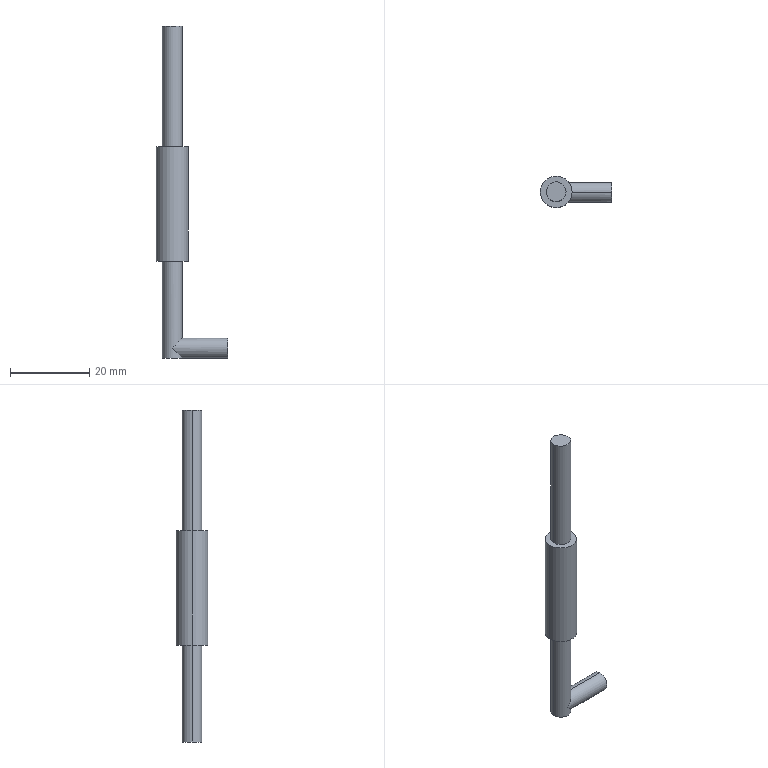Part | STEP file | HI_HFG87-17-002(2)^HFG87-17(2)_Lower机架DoorPlate 2 | 1 solid | 13 faces | box 18 x 8 x 84 mm | volume 2771 mm3 | cylinder 8 | plane 5 | commonest cylinder face diameters 5 x6 8 x2
STEP:
#1=CARTESIAN_POINT('',(0.,0.,0.));
#2=DIRECTION('',(0.,0.,1.));
#3=DIRECTION('',(1.,0.,0.));
#4=AXIS2_PLACEMENT_3D('',#1,#2,#3);
#5=CARTESIAN_POINT('',(-2.5,0.,44.5));
#6=VERTEX_POINT('',#5);
#7=CARTESIAN_POINT('',(2.5,0.,44.5));
#8=VERTEX_POINT('',#7);
#9=CARTESIAN_POINT('',(0.,0.,44.5));
#10=DIRECTION('',(0.,0.,1.));
#11=DIRECTION('',(1.,0.,0.));
#12=AXIS2_PLACEMENT_3D('',#9,#10,#11);
#13=CIRCLE('',#12,2.5);
#14=CARTESIAN_POINT('',(0.,0.,75.));
#15=DIRECTION('',(0.,0.,1.));
#16=DIRECTION('',(-1.,0.,0.));
#17=AXIS2_PLACEMENT_3D('',#14,#15,#16);
#18=CYLINDRICAL_SURFACE('',#17,2.5);
#19=CARTESIAN_POINT('',(-3.142,-30.5));
#20=DIRECTION('',(1.,0.));
#21=VECTOR('',#20,1.);
#22=LINE('',#19,#21);
#23=(GEOMETRIC_REPRESENTATION_CONTEXT(2)PARAMETRIC_REPRESENTATION_CONTEXT()REPRESENTATION_CONTEXT('',''));
#24=DEFINITIONAL_REPRESENTATION('',(#22),#23);
#25=PCURVE('',#18,#24);
#26=CARTESIAN_POINT('',(0.,0.,44.5));
#27=DIRECTION('',(0.,0.,1.));
#28=DIRECTION('',(1.,0.,0.));
#29=AXIS2_PLACEMENT_3D('',#26,#27,#28);
#30=PLANE('',#29);
#31=CARTESIAN_POINT('',(0.,0.));
#32=DIRECTION('',(1.,0.));
#33=AXIS2_PLACEMENT_2D('',#31,#32);
#34=CIRCLE('',#33,2.5);
#35=(GEOMETRIC_REPRESENTATION_CONTEXT(2)PARAMETRIC_REPRESENTATION_CONTEXT()REPRESENTATION_CONTEXT('',''));
#36=DEFINITIONAL_REPRESENTATION('',(#34),#35);
#37=PCURVE('',#30,#36);
#38=SURFACE_CURVE('',#13,(#25,#37),.PCURVE_S1.);
#39=EDGE_CURVE('',#6,#8,#38,.T.);
#40=ORIENTED_EDGE('',*,*,#39,.T.);
#41=CARTESIAN_POINT('',(2.5,0.,75.));
#42=VERTEX_POINT('',#41);
#43=CARTESIAN_POINT('',(2.5,0.,75.));
#44=DIRECTION('',(0.,0.,1.));
#45=VECTOR('',#44,1.);
#46=LINE('',#43,#45);
#47=CARTESIAN_POINT('',(3.142,0.));
#48=DIRECTION('',(0.,1.));
#49=VECTOR('',#48,1.);
#50=LINE('',#47,#49);
#51=(GEOMETRIC_REPRESENTATION_CONTEXT(2)PARAMETRIC_REPRESENTATION_CONTEXT()REPRESENTATION_CONTEXT('',''));
#52=DEFINITIONAL_REPRESENTATION('',(#50),#51);
#53=PCURVE('',#18,#52);
#54=CARTESIAN_POINT('',(0.,0.,75.));
#55=DIRECTION('',(0.,0.,1.));
#56=DIRECTION('',(-1.,0.,0.));
#57=AXIS2_PLACEMENT_3D('',#54,#55,#56);
#58=CYLINDRICAL_SURFACE('',#57,2.5);
#59=CARTESIAN_POINT('',(3.142,0.));
#60=DIRECTION('',(0.,1.));
#61=VECTOR('',#60,1.);
#62=LINE('',#59,#61);
#63=(GEOMETRIC_REPRESENTATION_CONTEXT(2)PARAMETRIC_REPRESENTATION_CONTEXT()REPRESENTATION_CONTEXT('',''));
#64=DEFINITIONAL_REPRESENTATION('',(#62),#63);
#65=PCURVE('',#58,#64);
#66=SURFACE_CURVE('',#46,(#53,#65),.PCURVE_S1.);
#67=EDGE_CURVE('',#8,#42,#66,.T.);
#68=ORIENTED_EDGE('',*,*,#67,.T.);
#69=CARTESIAN_POINT('',(-2.5,0.,75.));
#70=VERTEX_POINT('',#69);
#71=CARTESIAN_POINT('',(0.,0.,75.));
#72=DIRECTION('',(0.,0.,1.));
#73=DIRECTION('',(1.,0.,0.));
#74=AXIS2_PLACEMENT_3D('',#71,#72,#73);
#75=CIRCLE('',#74,2.5);
#76=CARTESIAN_POINT('',(-3.142,0.));
#77=DIRECTION('',(1.,0.));
#78=VECTOR('',#77,1.);
#79=LINE('',#76,#78);
#80=(GEOMETRIC_REPRESENTATION_CONTEXT(2)PARAMETRIC_REPRESENTATION_CONTEXT()REPRESENTATION_CONTEXT('',''));
#81=DEFINITIONAL_REPRESENTATION('',(#79),#80);
#82=PCURVE('',#18,#81);
#83=CARTESIAN_POINT('',(0.,0.,75.));
#84=DIRECTION('',(0.,0.,1.));
#85=DIRECTION('',(1.,0.,0.));
#86=AXIS2_PLACEMENT_3D('',#83,#84,#85);
#87=PLANE('',#86);
#88=CARTESIAN_POINT('',(0.,0.));
#89=DIRECTION('',(1.,0.));
#90=AXIS2_PLACEMENT_2D('',#88,#89);
#91=CIRCLE('',#90,2.5);
#92=(GEOMETRIC_REPRESENTATION_CONTEXT(2)PARAMETRIC_REPRESENTATION_CONTEXT()REPRESENTATION_CONTEXT('',''));
#93=DEFINITIONAL_REPRESENTATION('',(#91),#92);
#94=PCURVE('',#87,#93);
#95=SURFACE_CURVE('',#75,(#82,#94),.PCURVE_S1.);
#96=EDGE_CURVE('',#70,#42,#95,.T.);
#97=ORIENTED_EDGE('',*,*,#96,.F.);
#98=CARTESIAN_POINT('',(-2.5,0.,75.));
#99=DIRECTION('',(0.,0.,1.));
#100=VECTOR('',#99,1.);
#101=LINE('',#98,#100);
#102=CARTESIAN_POINT('',(0.,0.));
#103=DIRECTION('',(0.,1.));
#104=VECTOR('',#103,1.);
#105=LINE('',#102,#104);
#106=(GEOMETRIC_REPRESENTATION_CONTEXT(2)PARAMETRIC_REPRESENTATION_CONTEXT()REPRESENTATION_CONTEXT('',''));
#107=DEFINITIONAL_REPRESENTATION('',(#105),#106);
#108=PCURVE('',#18,#107);
#109=CARTESIAN_POINT('',(6.283,0.));
#110=DIRECTION('',(0.,1.));
#111=VECTOR('',#110,1.);
#112=LINE('',#109,#111);
#113=(GEOMETRIC_REPRESENTATION_CONTEXT(2)PARAMETRIC_REPRESENTATION_CONTEXT()REPRESENTATION_CONTEXT('',''));
#114=DEFINITIONAL_REPRESENTATION('',(#112),#113);
#115=PCURVE('',#58,#114);
#116=SURFACE_CURVE('',#101,(#108,#115),.PCURVE_S1.);
#117=EDGE_CURVE('',#6,#70,#116,.T.);
#118=ORIENTED_EDGE('',*,*,#117,.F.);
#119=EDGE_LOOP('',(#40,#68,#97,#118));
#120=FACE_BOUND('',#119,.T.);
#121=ADVANCED_FACE('',(#120),#18,.T.);
#122=CARTESIAN_POINT('',(2.5,0.,-4.));
#123=VERTEX_POINT('',#122);
#124=CARTESIAN_POINT('',(0.,-2.5,-6.5));
#125=VERTEX_POINT('',#124);
#126=CARTESIAN_POINT('',(2.5,0.,-4.));
#127=CARTESIAN_POINT('',(2.5,-1.464,-4.));
#128=CARTESIAN_POINT('',(1.464,-2.5,-5.036));
#129=CARTESIAN_POINT('',(0.,-2.5,-6.5));
#130=(BOUNDED_CURVE()B_SPLINE_CURVE(3,(#126,#127,#128,#129),.UNSPECIFIED.,.F.,.F.)B_SPLINE_CURVE_WITH_KNOTS((4,4),(3.142,4.712),.PIECEWISE_BEZIER_KNOTS.)CURVE()GEOMETRIC_REPRESENTATION_ITEM()RATIONAL_B_SPLINE_CURVE((1.,0.8047,0.8047,1.))REPRESENTATION_ITEM(''));
#131=CARTESIAN_POINT('',(0.,0.,75.));
#132=DIRECTION('',(0.,0.,1.));
#133=DIRECTION('',(-1.,0.,0.));
#134=AXIS2_PLACEMENT_3D('',#131,#132,#133);
#135=CYLINDRICAL_SURFACE('',#134,2.5);
#136=CARTESIAN_POINT('',(3.142,-79.));
#137=CARTESIAN_POINT('',(3.12,-79.));
#138=CARTESIAN_POINT('',(3.077,-79.003));
#139=CARTESIAN_POINT('',(3.01,-79.02));
#140=CARTESIAN_POINT('',(2.942,-79.048));
#141=CARTESIAN_POINT('',(2.872,-79.088));
#142=CARTESIAN_POINT('',(2.801,-79.142));
#143=CARTESIAN_POINT('',(2.729,-79.208));
#144=CARTESIAN_POINT('',(2.655,-79.288));
#145=CARTESIAN_POINT('',(2.581,-79.38));
#146=CARTESIAN_POINT('',(2.507,-79.485));
#147=CARTESIAN_POINT('',(2.432,-79.602));
#148=CARTESIAN_POINT('',(2.356,-79.731));
#149=CARTESIAN_POINT('',(2.281,-79.869));
#150=CARTESIAN_POINT('',(2.206,-80.016));
#151=CARTESIAN_POINT('',(2.131,-80.17));
#152=CARTESIAN_POINT('',(2.057,-80.331));
#153=CARTESIAN_POINT('',(1.984,-80.496));
#154=CARTESIAN_POINT('',(1.912,-80.664));
#155=CARTESIAN_POINT('',(1.841,-80.833));
#156=CARTESIAN_POINT('',(1.771,-81.003));
#157=CARTESIAN_POINT('',(1.702,-81.172));
#158=CARTESIAN_POINT('',(1.636,-81.338));
#159=CARTESIAN_POINT('',(1.592,-81.446));
#160=CARTESIAN_POINT('',(1.571,-81.5));
#161=B_SPLINE_CURVE_WITH_KNOTS('',3,(#136,#137,#138,#139,#140,#141,#142,#143,#144,#145,#146,#147,#148,#149,#150,#151,#152,#153,#154,#155,#156,#157,#158,#159,#160),.UNSPECIFIED.,.F.,.F.,(4,1,1,1,1,1,1,1,1,1,1,1,1,1,1,1,1,1,1,1,1,1,4),(3.142,3.213,3.284,3.356,3.427,3.499,3.57,3.641,3.713,3.784,3.856,3.927,3.998,4.07,4.141,4.213,4.284,4.355,4.427,4.498,4.57,4.641,4.712),.QUASI_UNIFORM_KNOTS.);
#162=(GEOMETRIC_REPRESENTATION_CONTEXT(2)PARAMETRIC_REPRESENTATION_CONTEXT()REPRESENTATION_CONTEXT('',''));
#163=DEFINITIONAL_REPRESENTATION('',(#161),#162);
#164=PCURVE('',#135,#163);
#165=CARTESIAN_POINT('',(14.,0.,-6.5));
#166=DIRECTION('',(-1.,0.,0.));
#167=DIRECTION('',(0.,0.,-1.));
#168=AXIS2_PLACEMENT_3D('',#165,#166,#167);
#169=CYLINDRICAL_SURFACE('',#168,2.5);
#170=CARTESIAN_POINT('',(3.142,11.5));
#171=CARTESIAN_POINT('',(3.12,11.5));
#172=CARTESIAN_POINT('',(3.077,11.503));
#173=CARTESIAN_POINT('',(3.01,11.52));
#174=CARTESIAN_POINT('',(2.942,11.548));
#175=CARTESIAN_POINT('',(2.872,11.588));
#176=CARTESIAN_POINT('',(2.801,11.642));
#177=CARTESIAN_POINT('',(2.729,11.708));
#178=CARTESIAN_POINT('',(2.655,11.788));
#179=CARTESIAN_POINT('',(2.581,11.88));
#180=CARTESIAN_POINT('',(2.507,11.985));
#181=CARTESIAN_POINT('',(2.432,12.102));
#182=CARTESIAN_POINT('',(2.356,12.231));
#183=CARTESIAN_POINT('',(2.281,12.369));
#184=CARTESIAN_POINT('',(2.206,12.516));
#185=CARTESIAN_POINT('',(2.131,12.67));
#186=CARTESIAN_POINT('',(2.057,12.831));
#187=CARTESIAN_POINT('',(1.984,12.996));
#188=CARTESIAN_POINT('',(1.912,13.164));
#189=CARTESIAN_POINT('',(1.841,13.333));
#190=CARTESIAN_POINT('',(1.771,13.503));
#191=CARTESIAN_POINT('',(1.702,13.672));
#192=CARTESIAN_POINT('',(1.636,13.838));
#193=CARTESIAN_POINT('',(1.592,13.946));
#194=CARTESIAN_POINT('',(1.571,14.));
#195=B_SPLINE_CURVE_WITH_KNOTS('',3,(#170,#171,#172,#173,#174,#175,#176,#177,#178,#179,#180,#181,#182,#183,#184,#185,#186,#187,#188,#189,#190,#191,#192,#193,#194),.UNSPECIFIED.,.F.,.F.,(4,1,1,1,1,1,1,1,1,1,1,1,1,1,1,1,1,1,1,1,1,1,4),(3.142,3.213,3.284,3.356,3.427,3.499,3.57,3.641,3.713,3.784,3.856,3.927,3.998,4.07,4.141,4.213,4.284,4.355,4.427,4.498,4.57,4.641,4.712),.QUASI_UNIFORM_KNOTS.);
#196=(GEOMETRIC_REPRESENTATION_CONTEXT(2)PARAMETRIC_REPRESENTATION_CONTEXT()REPRESENTATION_CONTEXT('',''));
#197=DEFINITIONAL_REPRESENTATION('',(#195),#196);
#198=PCURVE('',#169,#197);
#199=SURFACE_CURVE('',#130,(#164,#198),.PCURVE_S1.);
#200=EDGE_CURVE('',#123,#125,#199,.T.);
#201=ORIENTED_EDGE('',*,*,#200,.F.);
#202=CARTESIAN_POINT('',(2.5,0.,15.5));
#203=VERTEX_POINT('',#202);
#204=CARTESIAN_POINT('',(2.5,0.,75.));
#205=DIRECTION('',(0.,0.,1.));
#206=VECTOR('',#205,1.);
#207=LINE('',#204,#206);
#208=CARTESIAN_POINT('',(3.142,0.));
#209=DIRECTION('',(0.,1.));
#210=VECTOR('',#209,1.);
#211=LINE('',#208,#210);
#212=(GEOMETRIC_REPRESENTATION_CONTEXT(2)PARAMETRIC_REPRESENTATION_CONTEXT()REPRESENTATION_CONTEXT('',''));
#213=DEFINITIONAL_REPRESENTATION('',(#211),#212);
#214=PCURVE('',#135,#213);
#215=CARTESIAN_POINT('',(0.,0.,75.));
#216=DIRECTION('',(0.,0.,1.));
#217=DIRECTION('',(-1.,0.,0.));
#218=AXIS2_PLACEMENT_3D('',#215,#216,#217);
#219=CYLINDRICAL_SURFACE('',#218,2.5);
#220=CARTESIAN_POINT('',(3.142,0.));
#221=DIRECTION('',(0.,1.));
#222=VECTOR('',#221,1.);
#223=LINE('',#220,#222);
#224=(GEOMETRIC_REPRESENTATION_CONTEXT(2)PARAMETRIC_REPRESENTATION_CONTEXT()REPRESENTATION_CONTEXT('',''));
#225=DEFINITIONAL_REPRESENTATION('',(#223),#224);
#226=PCURVE('',#219,#225);
#227=SURFACE_CURVE('',#207,(#214,#226),.PCURVE_S1.);
#228=EDGE_CURVE('',#123,#203,#227,.T.);
#229=ORIENTED_EDGE('',*,*,#228,.T.);
#230=CARTESIAN_POINT('',(-2.5,0.,15.5));
#231=VERTEX_POINT('',#230);
#232=CARTESIAN_POINT('',(0.,0.,15.5));
#233=DIRECTION('',(0.,0.,1.));
#234=DIRECTION('',(1.,0.,0.));
#235=AXIS2_PLACEMENT_3D('',#232,#233,#234);
#236=CIRCLE('',#235,2.5);
#237=CARTESIAN_POINT('',(-3.142,-59.5));
#238=DIRECTION('',(1.,0.));
#239=VECTOR('',#238,1.);
#240=LINE('',#237,#239);
#241=(GEOMETRIC_REPRESENTATION_CONTEXT(2)PARAMETRIC_REPRESENTATION_CONTEXT()REPRESENTATION_CONTEXT('',''));
#242=DEFINITIONAL_REPRESENTATION('',(#240),#241);
#243=PCURVE('',#135,#242);
#244=CARTESIAN_POINT('',(0.,0.,15.5));
#245=DIRECTION('',(0.,0.,1.));
#246=DIRECTION('',(1.,0.,0.));
#247=AXIS2_PLACEMENT_3D('',#244,#245,#246);
#248=PLANE('',#247);
#249=CARTESIAN_POINT('',(0.,0.));
#250=DIRECTION('',(1.,0.));
#251=AXIS2_PLACEMENT_2D('',#249,#250);
#252=CIRCLE('',#251,2.5);
#253=(GEOMETRIC_REPRESENTATION_CONTEXT(2)PARAMETRIC_REPRESENTATION_CONTEXT()REPRESENTATION_CONTEXT('',''));
#254=DEFINITIONAL_REPRESENTATION('',(#252),#253);
#255=PCURVE('',#248,#254);
#256=SURFACE_CURVE('',#236,(#243,#255),.PCURVE_S1.);
#257=EDGE_CURVE('',#231,#203,#256,.T.);
#258=ORIENTED_EDGE('',*,*,#257,.F.);
#259=CARTESIAN_POINT('',(-2.5,0.,-9.));
#260=VERTEX_POINT('',#259);
#261=CARTESIAN_POINT('',(-2.5,0.,75.));
#262=DIRECTION('',(0.,0.,1.));
#263=VECTOR('',#262,1.);
#264=LINE('',#261,#263);
#265=CARTESIAN_POINT('',(0.,0.));
#266=DIRECTION('',(0.,1.));
#267=VECTOR('',#266,1.);
#268=LINE('',#265,#267);
#269=(GEOMETRIC_REPRESENTATION_CONTEXT(2)PARAMETRIC_REPRESENTATION_CONTEXT()REPRESENTATION_CONTEXT('',''));
#270=DEFINITIONAL_REPRESENTATION('',(#268),#269);
#271=PCURVE('',#135,#270);
#272=CARTESIAN_POINT('',(6.283,0.));
#273=DIRECTION('',(0.,1.));
#274=VECTOR('',#273,1.);
#275=LINE('',#272,#274);
#276=(GEOMETRIC_REPRESENTATION_CONTEXT(2)PARAMETRIC_REPRESENTATION_CONTEXT()REPRESENTATION_CONTEXT('',''));
#277=DEFINITIONAL_REPRESENTATION('',(#275),#276);
#278=PCURVE('',#219,#277);
#279=SURFACE_CURVE('',#264,(#271,#278),.PCURVE_S1.);
#280=EDGE_CURVE('',#260,#231,#279,.T.);
#281=ORIENTED_EDGE('',*,*,#280,.F.);
#282=CARTESIAN_POINT('',(2.5,0.,-9.));
#283=VERTEX_POINT('',#282);
#284=CARTESIAN_POINT('',(0.,0.,-9.));
#285=DIRECTION('',(0.,0.,1.));
#286=DIRECTION('',(1.,0.,0.));
#287=AXIS2_PLACEMENT_3D('',#284,#285,#286);
#288=CIRCLE('',#287,2.5);
#289=CARTESIAN_POINT('',(-3.142,-84.));
#290=DIRECTION('',(1.,0.));
#291=VECTOR('',#290,1.);
#292=LINE('',#289,#291);
#293=(GEOMETRIC_REPRESENTATION_CONTEXT(2)PARAMETRIC_REPRESENTATION_CONTEXT()REPRESENTATION_CONTEXT('',''));
#294=DEFINITIONAL_REPRESENTATION('',(#292),#293);
#295=PCURVE('',#135,#294);
#296=CARTESIAN_POINT('',(0.,0.,-9.));
#297=DIRECTION('',(0.,0.,1.));
#298=DIRECTION('',(1.,0.,0.));
#299=AXIS2_PLACEMENT_3D('',#296,#297,#298);
#300=PLANE('',#299);
#301=CARTESIAN_POINT('',(0.,0.));
#302=DIRECTION('',(1.,0.));
#303=AXIS2_PLACEMENT_2D('',#301,#302);
#304=CIRCLE('',#303,2.5);
#305=(GEOMETRIC_REPRESENTATION_CONTEXT(2)PARAMETRIC_REPRESENTATION_CONTEXT()REPRESENTATION_CONTEXT('',''));
#306=DEFINITIONAL_REPRESENTATION('',(#304),#305);
#307=PCURVE('',#300,#306);
#308=SURFACE_CURVE('',#288,(#295,#307),.PCURVE_S1.);
#309=EDGE_CURVE('',#260,#283,#308,.T.);
#310=ORIENTED_EDGE('',*,*,#309,.T.);
#311=CARTESIAN_POINT('',(0.,-2.5,-6.5));
#312=CARTESIAN_POINT('',(1.464,-2.5,-7.964));
#313=CARTESIAN_POINT('',(2.5,-1.464,-9.));
#314=CARTESIAN_POINT('',(2.5,0.,-9.));
#315=(BOUNDED_CURVE()B_SPLINE_CURVE(3,(#311,#312,#313,#314),.UNSPECIFIED.,.F.,.F.)B_SPLINE_CURVE_WITH_KNOTS((4,4),(4.712,6.283),.PIECEWISE_BEZIER_KNOTS.)CURVE()GEOMETRIC_REPRESENTATION_ITEM()RATIONAL_B_SPLINE_CURVE((1.,0.8047,0.8047,1.))REPRESENTATION_ITEM(''));
#316=CARTESIAN_POINT('',(1.571,-81.5));
#317=CARTESIAN_POINT('',(1.592,-81.554));
#318=CARTESIAN_POINT('',(1.636,-81.662));
#319=CARTESIAN_POINT('',(1.702,-81.828));
#320=CARTESIAN_POINT('',(1.771,-81.997));
#321=CARTESIAN_POINT('',(1.841,-82.167));
#322=CARTESIAN_POINT('',(1.912,-82.336));
#323=CARTESIAN_POINT('',(1.984,-82.504));
#324=CARTESIAN_POINT('',(2.057,-82.669));
#325=CARTESIAN_POINT('',(2.131,-82.83));
#326=CARTESIAN_POINT('',(2.206,-82.984));
#327=CARTESIAN_POINT('',(2.281,-83.131));
#328=CARTESIAN_POINT('',(2.356,-83.269));
#329=CARTESIAN_POINT('',(2.432,-83.398));
#330=CARTESIAN_POINT('',(2.507,-83.515));
#331=CARTESIAN_POINT('',(2.581,-83.62));
#332=CARTESIAN_POINT('',(2.655,-83.712));
#333=CARTESIAN_POINT('',(2.729,-83.792));
#334=CARTESIAN_POINT('',(2.801,-83.858));
#335=CARTESIAN_POINT('',(2.872,-83.912));
#336=CARTESIAN_POINT('',(2.942,-83.952));
#337=CARTESIAN_POINT('',(3.01,-83.98));
#338=CARTESIAN_POINT('',(3.077,-83.997));
#339=CARTESIAN_POINT('',(3.12,-84.));
#340=CARTESIAN_POINT('',(3.142,-84.));
#341=B_SPLINE_CURVE_WITH_KNOTS('',3,(#316,#317,#318,#319,#320,#321,#322,#323,#324,#325,#326,#327,#328,#329,#330,#331,#332,#333,#334,#335,#336,#337,#338,#339,#340),.UNSPECIFIED.,.F.,.F.,(4,1,1,1,1,1,1,1,1,1,1,1,1,1,1,1,1,1,1,1,1,1,4),(4.712,4.784,4.855,4.927,4.998,5.069,5.141,5.212,5.284,5.355,5.426,5.498,5.569,5.641,5.712,5.783,5.855,5.926,5.998,6.069,6.14,6.212,6.283),.QUASI_UNIFORM_KNOTS.);
#342=(GEOMETRIC_REPRESENTATION_CONTEXT(2)PARAMETRIC_REPRESENTATION_CONTEXT()REPRESENTATION_CONTEXT('',''));
#343=DEFINITIONAL_REPRESENTATION('',(#341),#342);
#344=PCURVE('',#135,#343);
#345=CARTESIAN_POINT('',(1.571,14.));
#346=CARTESIAN_POINT('',(1.549,13.946));
#347=CARTESIAN_POINT('',(1.506,13.838));
#348=CARTESIAN_POINT('',(1.439,13.672));
#349=CARTESIAN_POINT('',(1.371,13.503));
#350=CARTESIAN_POINT('',(1.301,13.333));
#351=CARTESIAN_POINT('',(1.23,13.164));
#352=CARTESIAN_POINT('',(1.158,12.996));
#353=CARTESIAN_POINT('',(1.085,12.831));
#354=CARTESIAN_POINT('',(1.01,12.67));
#355=CARTESIAN_POINT('',(0.9358,12.516));
#356=CARTESIAN_POINT('',(0.8607,12.369));
#357=CARTESIAN_POINT('',(0.7854,12.231));
#358=CARTESIAN_POINT('',(0.7101,12.102));
#359=CARTESIAN_POINT('',(0.635,11.985));
#360=CARTESIAN_POINT('',(0.5603,11.88));
#361=CARTESIAN_POINT('',(0.4863,11.788));
#362=CARTESIAN_POINT('',(0.413,11.708));
#363=CARTESIAN_POINT('',(0.3408,11.642));
#364=CARTESIAN_POINT('',(0.2697,11.588));
#365=CARTESIAN_POINT('',(0.2,11.548));
#366=CARTESIAN_POINT('',(0.1316,11.52));
#367=CARTESIAN_POINT('',(0.06485,11.503));
#368=CARTESIAN_POINT('',(0.02143,11.5));
#369=CARTESIAN_POINT('',(0.,11.5));
#370=B_SPLINE_CURVE_WITH_KNOTS('',3,(#345,#346,#347,#348,#349,#350,#351,#352,#353,#354,#355,#356,#357,#358,#359,#360,#361,#362,#363,#364,#365,#366,#367,#368,#369),.UNSPECIFIED.,.F.,.F.,(4,1,1,1,1,1,1,1,1,1,1,1,1,1,1,1,1,1,1,1,1,1,4),(4.712,4.784,4.855,4.927,4.998,5.069,5.141,5.212,5.284,5.355,5.426,5.498,5.569,5.641,5.712,5.783,5.855,5.926,5.998,6.069,6.14,6.212,6.283),.QUASI_UNIFORM_KNOTS.);
#371=(GEOMETRIC_REPRESENTATION_CONTEXT(2)PARAMETRIC_REPRESENTATION_CONTEXT()REPRESENTATION_CONTEXT('',''));
#372=DEFINITIONAL_REPRESENTATION('',(#370),#371);
#373=PCURVE('',#169,#372);
#374=SURFACE_CURVE('',#315,(#344,#373),.PCURVE_S1.);
#375=EDGE_CURVE('',#125,#283,#374,.T.);
#376=ORIENTED_EDGE('',*,*,#375,.F.);
#377=EDGE_LOOP('',(#201,#229,#258,#281,#310,#376));
#378=FACE_BOUND('',#377,.T.);
#379=ADVANCED_FACE('',(#378),#135,.T.);
#380=CARTESIAN_POINT('',(14.,0.,-4.));
#381=VERTEX_POINT('',#380);
#382=CARTESIAN_POINT('',(14.,0.,-9.));
#383=VERTEX_POINT('',#382);
#384=CARTESIAN_POINT('',(14.,0.,-6.5));
#385=DIRECTION('',(1.,0.,0.));
#386=DIRECTION('',(0.,0.,-1.));
#387=AXIS2_PLACEMENT_3D('',#384,#385,#386);
#388=CIRCLE('',#387,2.5);
#389=CARTESIAN_POINT('',(6.283,0.));
#390=DIRECTION('',(-1.,0.));
#391=VECTOR('',#390,1.);
#392=LINE('',#389,#391);
#393=(GEOMETRIC_REPRESENTATION_CONTEXT(2)PARAMETRIC_REPRESENTATION_CONTEXT()REPRESENTATION_CONTEXT('',''));
#394=DEFINITIONAL_REPRESENTATION('',(#392),#393);
#395=PCURVE('',#169,#394);
#396=CARTESIAN_POINT('',(14.,0.,-9.));
#397=DIRECTION('',(-1.,0.,0.));
#398=DIRECTION('',(0.,0.,1.));
#399=AXIS2_PLACEMENT_3D('',#396,#397,#398);
#400=PLANE('',#399);
#401=CARTESIAN_POINT('',(0.,0.));
#402=CARTESIAN_POINT('',(0.,4.33));
#403=CARTESIAN_POINT('',(3.75,2.165));
#404=CARTESIAN_POINT('',(7.5,0.));
#405=CARTESIAN_POINT('',(3.75,-2.165));
#406=CARTESIAN_POINT('',(0.,-4.33));
#407=CARTESIAN_POINT('',(0.,0.));
#408=(BOUNDED_CURVE()B_SPLINE_CURVE(2,(#401,#402,#403,#404,#405,#406,#407),.UNSPECIFIED.,.T.,.F.)B_SPLINE_CURVE_WITH_KNOTS((1,2,2,2,2,1),(-2.094,0.,2.094,4.189,6.283,8.378),.UNSPECIFIED.)CURVE()GEOMETRIC_REPRESENTATION_ITEM()RATIONAL_B_SPLINE_CURVE((1.,0.5,1.,0.5,1.,0.5,1.))REPRESENTATION_ITEM(''));
#409=(GEOMETRIC_REPRESENTATION_CONTEXT(2)PARAMETRIC_REPRESENTATION_CONTEXT()REPRESENTATION_CONTEXT('',''));
#410=DEFINITIONAL_REPRESENTATION('',(#408),#409);
#411=PCURVE('',#400,#410);
#412=SURFACE_CURVE('',#388,(#395,#411),.PCURVE_S1.);
#413=EDGE_CURVE('',#381,#383,#412,.T.);
#414=ORIENTED_EDGE('',*,*,#413,.F.);
#415=CARTESIAN_POINT('',(14.,0.,-4.));
#416=DIRECTION('',(-1.,0.,0.));
#417=VECTOR('',#416,1.);
#418=LINE('',#415,#417);
#419=CARTESIAN_POINT('',(3.142,0.));
#420=DIRECTION('',(0.,1.));
#421=VECTOR('',#420,1.);
#422=LINE('',#419,#421);
#423=(GEOMETRIC_REPRESENTATION_CONTEXT(2)PARAMETRIC_REPRESENTATION_CONTEXT()REPRESENTATION_CONTEXT('',''));
#424=DEFINITIONAL_REPRESENTATION('',(#422),#423);
#425=PCURVE('',#169,#424);
#426=CARTESIAN_POINT('',(14.,0.,-6.5));
#427=DIRECTION('',(-1.,0.,0.));
#428=DIRECTION('',(0.,0.,-1.));
#429=AXIS2_PLACEMENT_3D('',#426,#427,#428);
#430=CYLINDRICAL_SURFACE('',#429,2.5);
#431=CARTESIAN_POINT('',(3.142,0.));
#432=DIRECTION('',(0.,1.));
#433=VECTOR('',#432,1.);
#434=LINE('',#431,#433);
#435=(GEOMETRIC_REPRESENTATION_CONTEXT(2)PARAMETRIC_REPRESENTATION_CONTEXT()REPRESENTATION_CONTEXT('',''));
#436=DEFINITIONAL_REPRESENTATION('',(#434),#435);
#437=PCURVE('',#430,#436);
#438=SURFACE_CURVE('',#418,(#425,#437),.PCURVE_S1.);
#439=EDGE_CURVE('',#381,#123,#438,.T.);
#440=ORIENTED_EDGE('',*,*,#439,.T.);
#441=ORIENTED_EDGE('',*,*,#200,.T.);
#442=ORIENTED_EDGE('',*,*,#375,.T.);
#443=CARTESIAN_POINT('',(14.,0.,-9.));
#444=DIRECTION('',(-1.,0.,0.));
#445=VECTOR('',#444,1.);
#446=LINE('',#443,#445);
#447=CARTESIAN_POINT('',(0.,0.));
#448=DIRECTION('',(0.,1.));
#449=VECTOR('',#448,1.);
#450=LINE('',#447,#449);
#451=(GEOMETRIC_REPRESENTATION_CONTEXT(2)PARAMETRIC_REPRESENTATION_CONTEXT()REPRESENTATION_CONTEXT('',''));
#452=DEFINITIONAL_REPRESENTATION('',(#450),#451);
#453=PCURVE('',#169,#452);
#454=CARTESIAN_POINT('',(6.283,0.));
#455=DIRECTION('',(0.,1.));
#456=VECTOR('',#455,1.);
#457=LINE('',#454,#456);
#458=(GEOMETRIC_REPRESENTATION_CONTEXT(2)PARAMETRIC_REPRESENTATION_CONTEXT()REPRESENTATION_CONTEXT('',''));
#459=DEFINITIONAL_REPRESENTATION('',(#457),#458);
#460=PCURVE('',#430,#459);
#461=SURFACE_CURVE('',#446,(#453,#460),.PCURVE_S1.);
#462=EDGE_CURVE('',#383,#283,#461,.T.);
#463=ORIENTED_EDGE('',*,*,#462,.F.);
#464=EDGE_LOOP('',(#414,#440,#441,#442,#463));
#465=FACE_BOUND('',#464,.T.);
#466=ADVANCED_FACE('',(#465),#169,.T.);
#467=CARTESIAN_POINT('',(-4.,0.,15.5));
#468=VERTEX_POINT('',#467);
#469=CARTESIAN_POINT('',(4.,0.,15.5));
#470=VERTEX_POINT('',#469);
#471=CARTESIAN_POINT('',(0.,0.,15.5));
#472=DIRECTION('',(0.,0.,1.));
#473=DIRECTION('',(1.,0.,0.));
#474=AXIS2_PLACEMENT_3D('',#471,#472,#473);
#475=CIRCLE('',#474,4.);
#476=CARTESIAN_POINT('',(0.,0.,44.5));
#477=DIRECTION('',(0.,0.,1.));
#478=DIRECTION('',(-1.,0.,0.));
#479=AXIS2_PLACEMENT_3D('',#476,#477,#478);
#480=CYLINDRICAL_SURFACE('',#479,4.);
#481=CARTESIAN_POINT('',(-3.142,-29.));
#482=DIRECTION('',(1.,0.));
#483=VECTOR('',#482,1.);
#484=LINE('',#481,#483);
#485=(GEOMETRIC_REPRESENTATION_CONTEXT(2)PARAMETRIC_REPRESENTATION_CONTEXT()REPRESENTATION_CONTEXT('',''));
#486=DEFINITIONAL_REPRESENTATION('',(#484),#485);
#487=PCURVE('',#480,#486);
#488=CARTESIAN_POINT('',(0.,0.));
#489=DIRECTION('',(1.,0.));
#490=AXIS2_PLACEMENT_2D('',#488,#489);
#491=CIRCLE('',#490,4.);
#492=(GEOMETRIC_REPRESENTATION_CONTEXT(2)PARAMETRIC_REPRESENTATION_CONTEXT()REPRESENTATION_CONTEXT('',''));
#493=DEFINITIONAL_REPRESENTATION('',(#491),#492);
#494=PCURVE('',#248,#493);
#495=SURFACE_CURVE('',#475,(#487,#494),.PCURVE_S1.);
#496=EDGE_CURVE('',#468,#470,#495,.T.);
#497=ORIENTED_EDGE('',*,*,#496,.T.);
#498=CARTESIAN_POINT('',(4.,0.,44.5));
#499=VERTEX_POINT('',#498);
#500=CARTESIAN_POINT('',(4.,0.,44.5));
#501=DIRECTION('',(0.,0.,1.));
#502=VECTOR('',#501,1.);
#503=LINE('',#500,#502);
#504=CARTESIAN_POINT('',(3.142,0.));
#505=DIRECTION('',(0.,1.));
#506=VECTOR('',#505,1.);
#507=LINE('',#504,#506);
#508=(GEOMETRIC_REPRESENTATION_CONTEXT(2)PARAMETRIC_REPRESENTATION_CONTEXT()REPRESENTATION_CONTEXT('',''));
#509=DEFINITIONAL_REPRESENTATION('',(#507),#508);
#510=PCURVE('',#480,#509);
#511=CARTESIAN_POINT('',(0.,0.,44.5));
#512=DIRECTION('',(0.,0.,1.));
#513=DIRECTION('',(-1.,0.,0.));
#514=AXIS2_PLACEMENT_3D('',#511,#512,#513);
#515=CYLINDRICAL_SURFACE('',#514,4.);
#516=CARTESIAN_POINT('',(3.142,0.));
#517=DIRECTION('',(0.,1.));
#518=VECTOR('',#517,1.);
#519=LINE('',#516,#518);
#520=(GEOMETRIC_REPRESENTATION_CONTEXT(2)PARAMETRIC_REPRESENTATION_CONTEXT()REPRESENTATION_CONTEXT('',''));
#521=DEFINITIONAL_REPRESENTATION('',(#519),#520);
#522=PCURVE('',#515,#521);
#523=SURFACE_CURVE('',#503,(#510,#522),.PCURVE_S1.);
#524=EDGE_CURVE('',#470,#499,#523,.T.);
#525=ORIENTED_EDGE('',*,*,#524,.T.);
#526=CARTESIAN_POINT('',(-4.,0.,44.5));
#527=VERTEX_POINT('',#526);
#528=CARTESIAN_POINT('',(0.,0.,44.5));
#529=DIRECTION('',(0.,0.,1.));
#530=DIRECTION('',(1.,0.,0.));
#531=AXIS2_PLACEMENT_3D('',#528,#529,#530);
#532=CIRCLE('',#531,4.);
#533=CARTESIAN_POINT('',(-3.142,0.));
#534=DIRECTION('',(1.,0.));
#535=VECTOR('',#534,1.);
#536=LINE('',#533,#535);
#537=(GEOMETRIC_REPRESENTATION_CONTEXT(2)PARAMETRIC_REPRESENTATION_CONTEXT()REPRESENTATION_CONTEXT('',''));
#538=DEFINITIONAL_REPRESENTATION('',(#536),#537);
#539=PCURVE('',#480,#538);
#540=CARTESIAN_POINT('',(0.,0.));
#541=DIRECTION('',(1.,0.));
#542=AXIS2_PLACEMENT_2D('',#540,#541);
#543=CIRCLE('',#542,4.);
#544=(GEOMETRIC_REPRESENTATION_CONTEXT(2)PARAMETRIC_REPRESENTATION_CONTEXT()REPRESENTATION_CONTEXT('',''));
#545=DEFINITIONAL_REPRESENTATION('',(#543),#544);
#546=PCURVE('',#30,#545);
#547=SURFACE_CURVE('',#532,(#539,#546),.PCURVE_S1.);
#548=EDGE_CURVE('',#527,#499,#547,.T.);
#549=ORIENTED_EDGE('',*,*,#548,.F.);
#550=CARTESIAN_POINT('',(-4.,0.,44.5));
#551=DIRECTION('',(0.,0.,1.));
#552=VECTOR('',#551,1.);
#553=LINE('',#550,#552);
#554=CARTESIAN_POINT('',(0.,0.));
#555=DIRECTION('',(0.,1.));
#556=VECTOR('',#555,1.);
#557=LINE('',#554,#556);
#558=(GEOMETRIC_REPRESENTATION_CONTEXT(2)PARAMETRIC_REPRESENTATION_CONTEXT()REPRESENTATION_CONTEXT('',''));
#559=DEFINITIONAL_REPRESENTATION('',(#557),#558);
#560=PCURVE('',#480,#559);
#561=CARTESIAN_POINT('',(6.283,0.));
#562=DIRECTION('',(0.,1.));
#563=VECTOR('',#562,1.);
#564=LINE('',#561,#563);
#565=(GEOMETRIC_REPRESENTATION_CONTEXT(2)PARAMETRIC_REPRESENTATION_CONTEXT()REPRESENTATION_CONTEXT('',''));
#566=DEFINITIONAL_REPRESENTATION('',(#564),#565);
#567=PCURVE('',#515,#566);
#568=SURFACE_CURVE('',#553,(#560,#567),.PCURVE_S1.);
#569=EDGE_CURVE('',#468,#527,#568,.T.);
#570=ORIENTED_EDGE('',*,*,#569,.F.);
#571=EDGE_LOOP('',(#497,#525,#549,#570));
#572=FACE_BOUND('',#571,.T.);
#573=ADVANCED_FACE('',(#572),#480,.T.);
#574=ORIENTED_EDGE('',*,*,#96,.T.);
#575=CARTESIAN_POINT('',(0.,0.,75.));
#576=DIRECTION('',(0.,0.,1.));
#577=DIRECTION('',(1.,0.,0.));
#578=AXIS2_PLACEMENT_3D('',#575,#576,#577);
#579=CIRCLE('',#578,2.5);
#580=CARTESIAN_POINT('',(0.,0.));
#581=DIRECTION('',(1.,0.));
#582=AXIS2_PLACEMENT_2D('',#580,#581);
#583=CIRCLE('',#582,2.5);
#584=(GEOMETRIC_REPRESENTATION_CONTEXT(2)PARAMETRIC_REPRESENTATION_CONTEXT()REPRESENTATION_CONTEXT('',''));
#585=DEFINITIONAL_REPRESENTATION('',(#583),#584);
#586=PCURVE('',#87,#585);
#587=CARTESIAN_POINT('',(3.142,0.));
#588=DIRECTION('',(1.,0.));
#589=VECTOR('',#588,1.);
#590=LINE('',#587,#589);
#591=(GEOMETRIC_REPRESENTATION_CONTEXT(2)PARAMETRIC_REPRESENTATION_CONTEXT()REPRESENTATION_CONTEXT('',''));
#592=DEFINITIONAL_REPRESENTATION('',(#590),#591);
#593=PCURVE('',#58,#592);
#594=SURFACE_CURVE('',#579,(#586,#593),.PCURVE_S1.);
#595=EDGE_CURVE('',#42,#70,#594,.T.);
#596=ORIENTED_EDGE('',*,*,#595,.T.);
#597=EDGE_LOOP('',(#574,#596));
#598=FACE_BOUND('',#597,.T.);
#599=ADVANCED_FACE('',(#598),#87,.T.);
#600=ORIENTED_EDGE('',*,*,#524,.F.);
#601=CARTESIAN_POINT('',(0.,0.,15.5));
#602=DIRECTION('',(0.,0.,1.));
#603=DIRECTION('',(1.,0.,0.));
#604=AXIS2_PLACEMENT_3D('',#601,#602,#603);
#605=CIRCLE('',#604,4.);
#606=CARTESIAN_POINT('',(3.142,-29.));
#607=DIRECTION('',(1.,0.));
#608=VECTOR('',#607,1.);
#609=LINE('',#606,#608);
#610=(GEOMETRIC_REPRESENTATION_CONTEXT(2)PARAMETRIC_REPRESENTATION_CONTEXT()REPRESENTATION_CONTEXT('',''));
#611=DEFINITIONAL_REPRESENTATION('',(#609),#610);
#612=PCURVE('',#515,#611);
#613=CARTESIAN_POINT('',(0.,0.));
#614=DIRECTION('',(1.,0.));
#615=AXIS2_PLACEMENT_2D('',#613,#614);
#616=CIRCLE('',#615,4.);
#617=(GEOMETRIC_REPRESENTATION_CONTEXT(2)PARAMETRIC_REPRESENTATION_CONTEXT()REPRESENTATION_CONTEXT('',''));
#618=DEFINITIONAL_REPRESENTATION('',(#616),#617);
#619=PCURVE('',#248,#618);
#620=SURFACE_CURVE('',#605,(#612,#619),.PCURVE_S1.);
#621=EDGE_CURVE('',#470,#468,#620,.T.);
#622=ORIENTED_EDGE('',*,*,#621,.T.);
#623=ORIENTED_EDGE('',*,*,#569,.T.);
#624=CARTESIAN_POINT('',(0.,0.,44.5));
#625=DIRECTION('',(0.,0.,1.));
#626=DIRECTION('',(1.,0.,0.));
#627=AXIS2_PLACEMENT_3D('',#624,#625,#626);
#628=CIRCLE('',#627,4.);
#629=CARTESIAN_POINT('',(3.142,0.));
#630=DIRECTION('',(1.,0.));
#631=VECTOR('',#630,1.);
#632=LINE('',#629,#631);
#633=(GEOMETRIC_REPRESENTATION_CONTEXT(2)PARAMETRIC_REPRESENTATION_CONTEXT()REPRESENTATION_CONTEXT('',''));
#634=DEFINITIONAL_REPRESENTATION('',(#632),#633);
#635=PCURVE('',#515,#634);
#636=CARTESIAN_POINT('',(0.,0.));
#637=DIRECTION('',(1.,0.));
#638=AXIS2_PLACEMENT_2D('',#636,#637);
#639=CIRCLE('',#638,4.);
#640=(GEOMETRIC_REPRESENTATION_CONTEXT(2)PARAMETRIC_REPRESENTATION_CONTEXT()REPRESENTATION_CONTEXT('',''));
#641=DEFINITIONAL_REPRESENTATION('',(#639),#640);
#642=PCURVE('',#30,#641);
#643=SURFACE_CURVE('',#628,(#635,#642),.PCURVE_S1.);
#644=EDGE_CURVE('',#499,#527,#643,.T.);
#645=ORIENTED_EDGE('',*,*,#644,.F.);
#646=EDGE_LOOP('',(#600,#622,#623,#645));
#647=FACE_BOUND('',#646,.T.);
#648=ADVANCED_FACE('',(#647),#515,.T.);
#649=ORIENTED_EDGE('',*,*,#257,.T.);
#650=CARTESIAN_POINT('',(0.,0.,15.5));
#651=DIRECTION('',(0.,0.,1.));
#652=DIRECTION('',(1.,0.,0.));
#653=AXIS2_PLACEMENT_3D('',#650,#651,#652);
#654=CIRCLE('',#653,2.5);
#655=CARTESIAN_POINT('',(0.,0.));
#656=DIRECTION('',(1.,0.));
#657=AXIS2_PLACEMENT_2D('',#655,#656);
#658=CIRCLE('',#657,2.5);
#659=(GEOMETRIC_REPRESENTATION_CONTEXT(2)PARAMETRIC_REPRESENTATION_CONTEXT()REPRESENTATION_CONTEXT('',''));
#660=DEFINITIONAL_REPRESENTATION('',(#658),#659);
#661=PCURVE('',#248,#660);
#662=CARTESIAN_POINT('',(3.142,-59.5));
#663=DIRECTION('',(1.,0.));
#664=VECTOR('',#663,1.);
#665=LINE('',#662,#664);
#666=(GEOMETRIC_REPRESENTATION_CONTEXT(2)PARAMETRIC_REPRESENTATION_CONTEXT()REPRESENTATION_CONTEXT('',''));
#667=DEFINITIONAL_REPRESENTATION('',(#665),#666);
#668=PCURVE('',#219,#667);
#669=SURFACE_CURVE('',#654,(#661,#668),.PCURVE_S1.);
#670=EDGE_CURVE('',#203,#231,#669,.T.);
#671=ORIENTED_EDGE('',*,*,#670,.T.);
#672=EDGE_LOOP('',(#649,#671));
#673=FACE_BOUND('',#672,.T.);
#674=ORIENTED_EDGE('',*,*,#496,.F.);
#675=ORIENTED_EDGE('',*,*,#621,.F.);
#676=EDGE_LOOP('',(#674,#675));
#677=FACE_BOUND('',#676,.T.);
#678=ADVANCED_FACE('',(#673,#677),#248,.F.);
#679=CARTESIAN_POINT('',(14.,0.,-6.5));
#680=DIRECTION('',(1.,0.,0.));
#681=DIRECTION('',(0.,0.,-1.));
#682=AXIS2_PLACEMENT_3D('',#679,#680,#681);
#683=CIRCLE('',#682,2.5);
#684=CARTESIAN_POINT('',(0.,0.));
#685=CARTESIAN_POINT('',(0.,4.33));
#686=CARTESIAN_POINT('',(3.75,2.165));
#687=CARTESIAN_POINT('',(7.5,0.));
#688=CARTESIAN_POINT('',(3.75,-2.165));
#689=CARTESIAN_POINT('',(0.,-4.33));
#690=CARTESIAN_POINT('',(0.,0.));
#691=(BOUNDED_CURVE()B_SPLINE_CURVE(2,(#684,#685,#686,#687,#688,#689,#690),.UNSPECIFIED.,.T.,.F.)B_SPLINE_CURVE_WITH_KNOTS((1,2,2,2,2,1),(-2.094,0.,2.094,4.189,6.283,8.378),.UNSPECIFIED.)CURVE()GEOMETRIC_REPRESENTATION_ITEM()RATIONAL_B_SPLINE_CURVE((1.,0.5,1.,0.5,1.,0.5,1.))REPRESENTATION_ITEM(''));
#692=(GEOMETRIC_REPRESENTATION_CONTEXT(2)PARAMETRIC_REPRESENTATION_CONTEXT()REPRESENTATION_CONTEXT('',''));
#693=DEFINITIONAL_REPRESENTATION('',(#691),#692);
#694=PCURVE('',#400,#693);
#695=CARTESIAN_POINT('',(6.283,0.));
#696=DIRECTION('',(-1.,0.));
#697=VECTOR('',#696,1.);
#698=LINE('',#695,#697);
#699=(GEOMETRIC_REPRESENTATION_CONTEXT(2)PARAMETRIC_REPRESENTATION_CONTEXT()REPRESENTATION_CONTEXT('',''));
#700=DEFINITIONAL_REPRESENTATION('',(#698),#699);
#701=PCURVE('',#430,#700);
#702=SURFACE_CURVE('',#683,(#694,#701),.PCURVE_S1.);
#703=EDGE_CURVE('',#383,#381,#702,.T.);
#704=ORIENTED_EDGE('',*,*,#703,.T.);
#705=ORIENTED_EDGE('',*,*,#413,.T.);
#706=EDGE_LOOP('',(#704,#705));
#707=FACE_BOUND('',#706,.T.);
#708=ADVANCED_FACE('',(#707),#400,.F.);
#709=CARTESIAN_POINT('',(0.,0.,-9.));
#710=DIRECTION('',(0.,0.,1.));
#711=DIRECTION('',(1.,0.,0.));
#712=AXIS2_PLACEMENT_3D('',#709,#710,#711);
#713=CIRCLE('',#712,2.5);
#714=CARTESIAN_POINT('',(0.,0.));
#715=DIRECTION('',(1.,0.));
#716=AXIS2_PLACEMENT_2D('',#714,#715);
#717=CIRCLE('',#716,2.5);
#718=(GEOMETRIC_REPRESENTATION_CONTEXT(2)PARAMETRIC_REPRESENTATION_CONTEXT()REPRESENTATION_CONTEXT('',''));
#719=DEFINITIONAL_REPRESENTATION('',(#717),#718);
#720=PCURVE('',#300,#719);
#721=CARTESIAN_POINT('',(3.142,-84.));
#722=DIRECTION('',(1.,0.));
#723=VECTOR('',#722,1.);
#724=LINE('',#721,#723);
#725=(GEOMETRIC_REPRESENTATION_CONTEXT(2)PARAMETRIC_REPRESENTATION_CONTEXT()REPRESENTATION_CONTEXT('',''));
#726=DEFINITIONAL_REPRESENTATION('',(#724),#725);
#727=PCURVE('',#219,#726);
#728=SURFACE_CURVE('',#713,(#720,#727),.PCURVE_S1.);
#729=EDGE_CURVE('',#283,#260,#728,.T.);
#730=ORIENTED_EDGE('',*,*,#729,.F.);
#731=ORIENTED_EDGE('',*,*,#309,.F.);
#732=EDGE_LOOP('',(#730,#731));
#733=FACE_BOUND('',#732,.T.);
#734=ADVANCED_FACE('',(#733),#300,.F.);
#735=ORIENTED_EDGE('',*,*,#439,.F.);
#736=ORIENTED_EDGE('',*,*,#703,.F.);
#737=ORIENTED_EDGE('',*,*,#462,.T.);
#738=CARTESIAN_POINT('',(0.,2.5,-6.5));
#739=VERTEX_POINT('',#738);
#740=CARTESIAN_POINT('',(2.5,0.,-9.));
#741=CARTESIAN_POINT('',(2.5,1.464,-9.));
#742=CARTESIAN_POINT('',(1.464,2.5,-7.964));
#743=CARTESIAN_POINT('',(0.,2.5,-6.5));
#744=(BOUNDED_CURVE()B_SPLINE_CURVE(3,(#740,#741,#742,#743),.UNSPECIFIED.,.F.,.F.)B_SPLINE_CURVE_WITH_KNOTS((4,4),(0.,1.571),.PIECEWISE_BEZIER_KNOTS.)CURVE()GEOMETRIC_REPRESENTATION_ITEM()RATIONAL_B_SPLINE_CURVE((1.,0.8047,0.8047,1.))REPRESENTATION_ITEM(''));
#745=CARTESIAN_POINT('',(6.283,11.5));
#746=CARTESIAN_POINT('',(6.262,11.5));
#747=CARTESIAN_POINT('',(6.218,11.503));
#748=CARTESIAN_POINT('',(6.152,11.52));
#749=CARTESIAN_POINT('',(6.083,11.548));
#750=CARTESIAN_POINT('',(6.013,11.588));
#751=CARTESIAN_POINT('',(5.942,11.642));
#752=CARTESIAN_POINT('',(5.87,11.708));
#753=CARTESIAN_POINT('',(5.797,11.788));
#754=CARTESIAN_POINT('',(5.723,11.88));
#755=CARTESIAN_POINT('',(5.648,11.985));
#756=CARTESIAN_POINT('',(5.573,12.102));
#757=CARTESIAN_POINT('',(5.498,12.231));
#758=CARTESIAN_POINT('',(5.422,12.369));
#759=CARTESIAN_POINT('',(5.347,12.516));
#760=CARTESIAN_POINT('',(5.273,12.67));
#761=CARTESIAN_POINT('',(5.199,12.831));
#762=CARTESIAN_POINT('',(5.125,12.996));
#763=CARTESIAN_POINT('',(5.053,13.164));
#764=CARTESIAN_POINT('',(4.982,13.333));
#765=CARTESIAN_POINT('',(4.912,13.503));
#766=CARTESIAN_POINT('',(4.844,13.672));
#767=CARTESIAN_POINT('',(4.777,13.838));
#768=CARTESIAN_POINT('',(4.734,13.946));
#769=CARTESIAN_POINT('',(4.712,14.));
#770=B_SPLINE_CURVE_WITH_KNOTS('',3,(#745,#746,#747,#748,#749,#750,#751,#752,#753,#754,#755,#756,#757,#758,#759,#760,#761,#762,#763,#764,#765,#766,#767,#768,#769),.UNSPECIFIED.,.F.,.F.,(4,1,1,1,1,1,1,1,1,1,1,1,1,1,1,1,1,1,1,1,1,1,4),(0.,0.0714,0.1428,0.2142,0.2856,0.357,0.4284,0.4998,0.5712,0.6426,0.714,0.7854,0.8568,0.9282,0.9996,1.071,1.142,1.214,1.285,1.357,1.428,1.499,1.571),.QUASI_UNIFORM_KNOTS.);
#771=(GEOMETRIC_REPRESENTATION_CONTEXT(2)PARAMETRIC_REPRESENTATION_CONTEXT()REPRESENTATION_CONTEXT('',''));
#772=DEFINITIONAL_REPRESENTATION('',(#770),#771);
#773=PCURVE('',#430,#772);
#774=CARTESIAN_POINT('',(3.142,-84.));
#775=CARTESIAN_POINT('',(3.163,-84.));
#776=CARTESIAN_POINT('',(3.206,-83.997));
#777=CARTESIAN_POINT('',(3.273,-83.98));
#778=CARTESIAN_POINT('',(3.342,-83.952));
#779=CARTESIAN_POINT('',(3.411,-83.912));
#780=CARTESIAN_POINT('',(3.482,-83.858));
#781=CARTESIAN_POINT('',(3.555,-83.792));
#782=CARTESIAN_POINT('',(3.628,-83.712));
#783=CARTESIAN_POINT('',(3.702,-83.62));
#784=CARTESIAN_POINT('',(3.777,-83.515));
#785=CARTESIAN_POINT('',(3.852,-83.398));
#786=CARTESIAN_POINT('',(3.927,-83.269));
#787=CARTESIAN_POINT('',(4.002,-83.131));
#788=CARTESIAN_POINT('',(4.077,-82.984));
#789=CARTESIAN_POINT('',(4.152,-82.83));
#790=CARTESIAN_POINT('',(4.226,-82.669));
#791=CARTESIAN_POINT('',(4.299,-82.504));
#792=CARTESIAN_POINT('',(4.372,-82.336));
#793=CARTESIAN_POINT('',(4.443,-82.167));
#794=CARTESIAN_POINT('',(4.512,-81.997));
#795=CARTESIAN_POINT('',(4.581,-81.828));
#796=CARTESIAN_POINT('',(4.648,-81.662));
#797=CARTESIAN_POINT('',(4.691,-81.554));
#798=CARTESIAN_POINT('',(4.712,-81.5));
#799=B_SPLINE_CURVE_WITH_KNOTS('',3,(#774,#775,#776,#777,#778,#779,#780,#781,#782,#783,#784,#785,#786,#787,#788,#789,#790,#791,#792,#793,#794,#795,#796,#797,#798),.UNSPECIFIED.,.F.,.F.,(4,1,1,1,1,1,1,1,1,1,1,1,1,1,1,1,1,1,1,1,1,1,4),(0.,0.0714,0.1428,0.2142,0.2856,0.357,0.4284,0.4998,0.5712,0.6426,0.714,0.7854,0.8568,0.9282,0.9996,1.071,1.142,1.214,1.285,1.357,1.428,1.499,1.571),.QUASI_UNIFORM_KNOTS.);
#800=(GEOMETRIC_REPRESENTATION_CONTEXT(2)PARAMETRIC_REPRESENTATION_CONTEXT()REPRESENTATION_CONTEXT('',''));
#801=DEFINITIONAL_REPRESENTATION('',(#799),#800);
#802=PCURVE('',#219,#801);
#803=SURFACE_CURVE('',#744,(#773,#802),.PCURVE_S1.);
#804=EDGE_CURVE('',#283,#739,#803,.T.);
#805=ORIENTED_EDGE('',*,*,#804,.T.);
#806=CARTESIAN_POINT('',(0.,2.5,-6.5));
#807=CARTESIAN_POINT('',(1.464,2.5,-5.036));
#808=CARTESIAN_POINT('',(2.5,1.464,-4.));
#809=CARTESIAN_POINT('',(2.5,0.,-4.));
#810=(BOUNDED_CURVE()B_SPLINE_CURVE(3,(#806,#807,#808,#809),.UNSPECIFIED.,.F.,.F.)B_SPLINE_CURVE_WITH_KNOTS((4,4),(1.571,3.142),.PIECEWISE_BEZIER_KNOTS.)CURVE()GEOMETRIC_REPRESENTATION_ITEM()RATIONAL_B_SPLINE_CURVE((1.,0.8047,0.8047,1.))REPRESENTATION_ITEM(''));
#811=CARTESIAN_POINT('',(4.712,14.));
#812=CARTESIAN_POINT('',(4.691,13.946));
#813=CARTESIAN_POINT('',(4.648,13.838));
#814=CARTESIAN_POINT('',(4.581,13.672));
#815=CARTESIAN_POINT('',(4.512,13.503));
#816=CARTESIAN_POINT('',(4.443,13.333));
#817=CARTESIAN_POINT('',(4.372,13.164));
#818=CARTESIAN_POINT('',(4.299,12.996));
#819=CARTESIAN_POINT('',(4.226,12.831));
#820=CARTESIAN_POINT('',(4.152,12.67));
#821=CARTESIAN_POINT('',(4.077,12.516));
#822=CARTESIAN_POINT('',(4.002,12.369));
#823=CARTESIAN_POINT('',(3.927,12.231));
#824=CARTESIAN_POINT('',(3.852,12.102));
#825=CARTESIAN_POINT('',(3.777,11.985));
#826=CARTESIAN_POINT('',(3.702,11.88));
#827=CARTESIAN_POINT('',(3.628,11.788));
#828=CARTESIAN_POINT('',(3.555,11.708));
#829=CARTESIAN_POINT('',(3.482,11.642));
#830=CARTESIAN_POINT('',(3.411,11.588));
#831=CARTESIAN_POINT('',(3.342,11.548));
#832=CARTESIAN_POINT('',(3.273,11.52));
#833=CARTESIAN_POINT('',(3.206,11.503));
#834=CARTESIAN_POINT('',(3.163,11.5));
#835=CARTESIAN_POINT('',(3.142,11.5));
#836=B_SPLINE_CURVE_WITH_KNOTS('',3,(#811,#812,#813,#814,#815,#816,#817,#818,#819,#820,#821,#822,#823,#824,#825,#826,#827,#828,#829,#830,#831,#832,#833,#834,#835),.UNSPECIFIED.,.F.,.F.,(4,1,1,1,1,1,1,1,1,1,1,1,1,1,1,1,1,1,1,1,1,1,4),(1.571,1.642,1.714,1.785,1.856,1.928,1.999,2.071,2.142,2.213,2.285,2.356,2.428,2.499,2.57,2.642,2.713,2.785,2.856,2.927,2.999,3.07,3.142),.QUASI_UNIFORM_KNOTS.);
#837=(GEOMETRIC_REPRESENTATION_CONTEXT(2)PARAMETRIC_REPRESENTATION_CONTEXT()REPRESENTATION_CONTEXT('',''));
#838=DEFINITIONAL_REPRESENTATION('',(#836),#837);
#839=PCURVE('',#430,#838);
#840=CARTESIAN_POINT('',(4.712,-81.5));
#841=CARTESIAN_POINT('',(4.691,-81.446));
#842=CARTESIAN_POINT('',(4.648,-81.338));
#843=CARTESIAN_POINT('',(4.581,-81.172));
#844=CARTESIAN_POINT('',(4.512,-81.003));
#845=CARTESIAN_POINT('',(4.443,-80.833));
#846=CARTESIAN_POINT('',(4.372,-80.664));
#847=CARTESIAN_POINT('',(4.299,-80.496));
#848=CARTESIAN_POINT('',(4.226,-80.331));
#849=CARTESIAN_POINT('',(4.152,-80.17));
#850=CARTESIAN_POINT('',(4.077,-80.016));
#851=CARTESIAN_POINT('',(4.002,-79.869));
#852=CARTESIAN_POINT('',(3.927,-79.731));
#853=CARTESIAN_POINT('',(3.852,-79.602));
#854=CARTESIAN_POINT('',(3.777,-79.485));
#855=CARTESIAN_POINT('',(3.702,-79.38));
#856=CARTESIAN_POINT('',(3.628,-79.288));
#857=CARTESIAN_POINT('',(3.555,-79.208));
#858=CARTESIAN_POINT('',(3.482,-79.142));
#859=CARTESIAN_POINT('',(3.411,-79.088));
#860=CARTESIAN_POINT('',(3.342,-79.048));
#861=CARTESIAN_POINT('',(3.273,-79.02));
#862=CARTESIAN_POINT('',(3.206,-79.003));
#863=CARTESIAN_POINT('',(3.163,-79.));
#864=CARTESIAN_POINT('',(3.142,-79.));
#865=B_SPLINE_CURVE_WITH_KNOTS('',3,(#840,#841,#842,#843,#844,#845,#846,#847,#848,#849,#850,#851,#852,#853,#854,#855,#856,#857,#858,#859,#860,#861,#862,#863,#864),.UNSPECIFIED.,.F.,.F.,(4,1,1,1,1,1,1,1,1,1,1,1,1,1,1,1,1,1,1,1,1,1,4),(1.571,1.642,1.714,1.785,1.856,1.928,1.999,2.071,2.142,2.213,2.285,2.356,2.428,2.499,2.57,2.642,2.713,2.785,2.856,2.927,2.999,3.07,3.142),.QUASI_UNIFORM_KNOTS.);
#866=(GEOMETRIC_REPRESENTATION_CONTEXT(2)PARAMETRIC_REPRESENTATION_CONTEXT()REPRESENTATION_CONTEXT('',''));
#867=DEFINITIONAL_REPRESENTATION('',(#865),#866);
#868=PCURVE('',#219,#867);
#869=SURFACE_CURVE('',#810,(#839,#868),.PCURVE_S1.);
#870=EDGE_CURVE('',#739,#123,#869,.T.);
#871=ORIENTED_EDGE('',*,*,#870,.T.);
#872=EDGE_LOOP('',(#735,#736,#737,#805,#871));
#873=FACE_BOUND('',#872,.T.);
#874=ADVANCED_FACE('',(#873),#430,.T.);
#875=ORIENTED_EDGE('',*,*,#228,.F.);
#876=ORIENTED_EDGE('',*,*,#870,.F.);
#877=ORIENTED_EDGE('',*,*,#804,.F.);
#878=ORIENTED_EDGE('',*,*,#729,.T.);
#879=ORIENTED_EDGE('',*,*,#280,.T.);
#880=ORIENTED_EDGE('',*,*,#670,.F.);
#881=EDGE_LOOP('',(#875,#876,#877,#878,#879,#880));
#882=FACE_BOUND('',#881,.T.);
#883=ADVANCED_FACE('',(#882),#219,.T.);
#884=ORIENTED_EDGE('',*,*,#67,.F.);
#885=CARTESIAN_POINT('',(0.,0.,44.5));
#886=DIRECTION('',(0.,0.,1.));
#887=DIRECTION('',(1.,0.,0.));
#888=AXIS2_PLACEMENT_3D('',#885,#886,#887);
#889=CIRCLE('',#888,2.5);
#890=CARTESIAN_POINT('',(3.142,-30.5));
#891=DIRECTION('',(1.,0.));
#892=VECTOR('',#891,1.);
#893=LINE('',#890,#892);
#894=(GEOMETRIC_REPRESENTATION_CONTEXT(2)PARAMETRIC_REPRESENTATION_CONTEXT()REPRESENTATION_CONTEXT('',''));
#895=DEFINITIONAL_REPRESENTATION('',(#893),#894);
#896=PCURVE('',#58,#895);
#897=CARTESIAN_POINT('',(0.,0.));
#898=DIRECTION('',(1.,0.));
#899=AXIS2_PLACEMENT_2D('',#897,#898);
#900=CIRCLE('',#899,2.5);
#901=(GEOMETRIC_REPRESENTATION_CONTEXT(2)PARAMETRIC_REPRESENTATION_CONTEXT()REPRESENTATION_CONTEXT('',''));
#902=DEFINITIONAL_REPRESENTATION('',(#900),#901);
#903=PCURVE('',#30,#902);
#904=SURFACE_CURVE('',#889,(#896,#903),.PCURVE_S1.);
#905=EDGE_CURVE('',#8,#6,#904,.T.);
#906=ORIENTED_EDGE('',*,*,#905,.T.);
#907=ORIENTED_EDGE('',*,*,#117,.T.);
#908=ORIENTED_EDGE('',*,*,#595,.F.);
#909=EDGE_LOOP('',(#884,#906,#907,#908));
#910=FACE_BOUND('',#909,.T.);
#911=ADVANCED_FACE('',(#910),#58,.T.);
#912=ORIENTED_EDGE('',*,*,#39,.F.);
#913=ORIENTED_EDGE('',*,*,#905,.F.);
#914=EDGE_LOOP('',(#912,#913));
#915=FACE_BOUND('',#914,.T.);
#916=ORIENTED_EDGE('',*,*,#548,.T.);
#917=ORIENTED_EDGE('',*,*,#644,.T.);
#918=EDGE_LOOP('',(#916,#917));
#919=FACE_BOUND('',#918,.T.);
#920=ADVANCED_FACE('',(#915,#919),#30,.T.);
#921=CLOSED_SHELL('',(#121,#379,#466,#573,#599,#648,#678,#708,#734,#874,#883,#911,#920));
#922=MANIFOLD_SOLID_BREP('',#921);
#923=(LENGTH_UNIT()NAMED_UNIT(*)SI_UNIT(.MILLI.,.METRE.));
#924=UNCERTAINTY_MEASURE_WITH_UNIT(LENGTH_MEASURE(0.0000001),#923,'','');
#925=(NAMED_UNIT(*)PLANE_ANGLE_UNIT()SI_UNIT($,.RADIAN.));
#926=(NAMED_UNIT(*)SI_UNIT($,.STERADIAN.)SOLID_ANGLE_UNIT());
#927=(GEOMETRIC_REPRESENTATION_CONTEXT(3)GLOBAL_UNCERTAINTY_ASSIGNED_CONTEXT((#924))GLOBAL_UNIT_ASSIGNED_CONTEXT((#923,#925,#926))REPRESENTATION_CONTEXT('',''));
#928=ADVANCED_BREP_SHAPE_REPRESENTATION('',(#4,#922),#927);